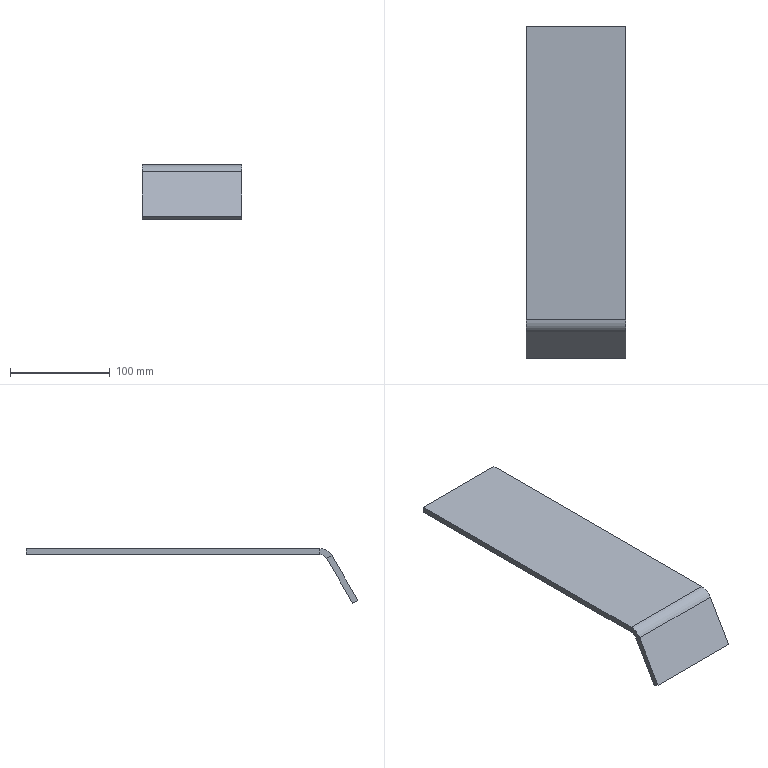Part | SolidWorks | features FlatPattern 1, SMBaseFlange 1, SheetMetal 1 | 1 solid | 14 faces | box 100 x 332 x 54.962 mm | volume 214412 mm3 | plane 12 | cylinder 2 | commonest cylinder face diameters 16 x1 28 x1
STEP:
#1=CARTESIAN_POINT('',(100.,8.083,0.));
#2=VERTEX_POINT('',#1);
#3=CARTESIAN_POINT('',(100.,8.083,-6.));
#4=VERTEX_POINT('',#3);
#5=CARTESIAN_POINT('',(100.,8.083,0.));
#6=DIRECTION('',(0.,0.,-1.));
#7=VECTOR('',#6,1000.);
#8=LINE('',#5,#7);
#9=EDGE_CURVE('',#2,#4,#8,.T.);
#10=ORIENTED_EDGE('',*,*,#9,.F.);
#11=CARTESIAN_POINT('',(100.,-4.041,-7.));
#12=VERTEX_POINT('',#11);
#13=CARTESIAN_POINT('',(100.,8.083,-14.));
#14=DIRECTION('',(1.,0.,0.));
#15=DIRECTION('',(0.,0.,1.));
#16=AXIS2_PLACEMENT_3D('',#13,#14,#15);
#17=CIRCLE('',#16,14.);
#18=EDGE_CURVE('',#2,#12,#17,.T.);
#19=ORIENTED_EDGE('',*,*,#18,.T.);
#20=CARTESIAN_POINT('',(100.,1.155,-10.));
#21=VERTEX_POINT('',#20);
#22=CARTESIAN_POINT('',(100.,1.155,-10.));
#23=DIRECTION('',(0.,-0.866,0.5));
#24=VECTOR('',#23,1000.);
#25=LINE('',#22,#24);
#26=EDGE_CURVE('',#21,#12,#25,.T.);
#27=ORIENTED_EDGE('',*,*,#26,.F.);
#28=CARTESIAN_POINT('',(100.,8.083,-14.));
#29=DIRECTION('',(1.,0.,0.));
#30=DIRECTION('',(0.,0.,-1.));
#31=AXIS2_PLACEMENT_3D('',#28,#29,#30);
#32=CIRCLE('',#31,8.);
#33=EDGE_CURVE('',#4,#21,#32,.T.);
#34=ORIENTED_EDGE('',*,*,#33,.F.);
#35=EDGE_LOOP('',(#10,#19,#27,#34));
#36=FACE_OUTER_BOUND('',#35,.T.);
#37=CARTESIAN_POINT('',(100.,8.083,0.));
#38=DIRECTION('',(1.,0.,0.));
#39=DIRECTION('',(0.,0.,-1.));
#40=AXIS2_PLACEMENT_3D('',#37,#38,#39);
#41=PLANE('',#40);
#42=ADVANCED_FACE('',(#36),#41,.T.);
#43=CARTESIAN_POINT('',(100.,302.,0.));
#44=VERTEX_POINT('',#43);
#45=CARTESIAN_POINT('',(100.,0.,0.));
#46=DIRECTION('',(0.,-1.,0.));
#47=VECTOR('',#46,1000.);
#48=LINE('',#45,#47);
#49=EDGE_CURVE('',#44,#2,#48,.T.);
#50=ORIENTED_EDGE('',*,*,#49,.T.);
#51=ORIENTED_EDGE('',*,*,#9,.T.);
#52=CARTESIAN_POINT('',(100.,302.,-6.));
#53=VERTEX_POINT('',#52);
#54=CARTESIAN_POINT('',(100.,0.,-6.));
#55=DIRECTION('',(0.,-1.,0.));
#56=VECTOR('',#55,1000.);
#57=LINE('',#54,#56);
#58=EDGE_CURVE('',#53,#4,#57,.T.);
#59=ORIENTED_EDGE('',*,*,#58,.F.);
#60=CARTESIAN_POINT('',(100.,302.,0.));
#61=DIRECTION('',(0.,0.,-1.));
#62=VECTOR('',#61,1000.);
#63=LINE('',#60,#62);
#64=EDGE_CURVE('',#44,#53,#63,.T.);
#65=ORIENTED_EDGE('',*,*,#64,.F.);
#66=EDGE_LOOP('',(#50,#51,#59,#65));
#67=FACE_OUTER_BOUND('',#66,.T.);
#68=CARTESIAN_POINT('',(100.,1.155,-10.));
#69=DIRECTION('',(1.,0.,0.));
#70=DIRECTION('',(0.,0.,-1.));
#71=AXIS2_PLACEMENT_3D('',#68,#69,#70);
#72=PLANE('',#71);
#73=ADVANCED_FACE('',(#67),#72,.T.);
#74=CARTESIAN_POINT('',(0.,-4.041,-7.));
#75=VERTEX_POINT('',#74);
#76=CARTESIAN_POINT('',(0.,1.155,-10.));
#77=VERTEX_POINT('',#76);
#78=CARTESIAN_POINT('',(0.,-4.041,-7.));
#79=DIRECTION('',(0.,0.866,-0.5));
#80=VECTOR('',#79,1000.);
#81=LINE('',#78,#80);
#82=EDGE_CURVE('',#75,#77,#81,.T.);
#83=ORIENTED_EDGE('',*,*,#82,.F.);
#84=CARTESIAN_POINT('',(0.,8.083,0.));
#85=VERTEX_POINT('',#84);
#86=CARTESIAN_POINT('',(0.,8.083,-14.));
#87=DIRECTION('',(1.,0.,0.));
#88=DIRECTION('',(0.,0.,1.));
#89=AXIS2_PLACEMENT_3D('',#86,#87,#88);
#90=CIRCLE('',#89,14.);
#91=EDGE_CURVE('',#85,#75,#90,.T.);
#92=ORIENTED_EDGE('',*,*,#91,.F.);
#93=CARTESIAN_POINT('',(0.,8.083,-6.));
#94=VERTEX_POINT('',#93);
#95=CARTESIAN_POINT('',(0.,8.083,-6.));
#96=DIRECTION('',(0.,0.,1.));
#97=VECTOR('',#96,1000.);
#98=LINE('',#95,#97);
#99=EDGE_CURVE('',#94,#85,#98,.T.);
#100=ORIENTED_EDGE('',*,*,#99,.F.);
#101=CARTESIAN_POINT('',(0.,8.083,-14.));
#102=DIRECTION('',(1.,0.,0.));
#103=DIRECTION('',(0.,0.,-1.));
#104=AXIS2_PLACEMENT_3D('',#101,#102,#103);
#105=CIRCLE('',#104,8.);
#106=EDGE_CURVE('',#94,#77,#105,.T.);
#107=ORIENTED_EDGE('',*,*,#106,.T.);
#108=EDGE_LOOP('',(#83,#92,#100,#107));
#109=FACE_OUTER_BOUND('',#108,.T.);
#110=CARTESIAN_POINT('',(0.,-4.041,-7.));
#111=DIRECTION('',(-1.,0.,0.));
#112=DIRECTION('',(0.,0.,1.));
#113=AXIS2_PLACEMENT_3D('',#110,#111,#112);
#114=PLANE('',#113);
#115=ADVANCED_FACE('',(#109),#114,.T.);
#116=CARTESIAN_POINT('',(0.,-30.,-51.962));
#117=VERTEX_POINT('',#116);
#118=CARTESIAN_POINT('',(0.,0.,0.));
#119=DIRECTION('',(0.,-0.5,-0.866));
#120=VECTOR('',#119,1000.);
#121=LINE('',#118,#120);
#122=EDGE_CURVE('',#75,#117,#121,.T.);
#123=ORIENTED_EDGE('',*,*,#122,.F.);
#124=ORIENTED_EDGE('',*,*,#82,.T.);
#125=CARTESIAN_POINT('',(0.,-24.804,-54.962));
#126=VERTEX_POINT('',#125);
#127=CARTESIAN_POINT('',(0.,5.196,-3.));
#128=DIRECTION('',(0.,-0.5,-0.866));
#129=VECTOR('',#128,1000.);
#130=LINE('',#127,#129);
#131=EDGE_CURVE('',#77,#126,#130,.T.);
#132=ORIENTED_EDGE('',*,*,#131,.T.);
#133=CARTESIAN_POINT('',(0.,-24.804,-54.962));
#134=DIRECTION('',(0.,-0.866,0.5));
#135=VECTOR('',#134,1000.);
#136=LINE('',#133,#135);
#137=EDGE_CURVE('',#126,#117,#136,.T.);
#138=ORIENTED_EDGE('',*,*,#137,.T.);
#139=EDGE_LOOP('',(#123,#124,#132,#138));
#140=FACE_OUTER_BOUND('',#139,.T.);
#141=CARTESIAN_POINT('',(0.,8.083,-6.));
#142=DIRECTION('',(-1.,0.,0.));
#143=DIRECTION('',(0.,0.,1.));
#144=AXIS2_PLACEMENT_3D('',#141,#142,#143);
#145=PLANE('',#144);
#146=ADVANCED_FACE('',(#140),#145,.T.);
#147=ORIENTED_EDGE('',*,*,#122,.T.);
#148=CARTESIAN_POINT('',(100.,-30.,-51.962));
#149=VERTEX_POINT('',#148);
#150=CARTESIAN_POINT('',(100.,-30.,-51.962));
#151=DIRECTION('',(-1.,0.,0.));
#152=VECTOR('',#151,1000.);
#153=LINE('',#150,#152);
#154=EDGE_CURVE('',#149,#117,#153,.T.);
#155=ORIENTED_EDGE('',*,*,#154,.F.);
#156=CARTESIAN_POINT('',(100.,0.,0.));
#157=DIRECTION('',(0.,-0.5,-0.866));
#158=VECTOR('',#157,1000.);
#159=LINE('',#156,#158);
#160=EDGE_CURVE('',#12,#149,#159,.T.);
#161=ORIENTED_EDGE('',*,*,#160,.F.);
#162=CARTESIAN_POINT('',(100.,-4.041,-7.));
#163=DIRECTION('',(-1.,0.,0.));
#164=VECTOR('',#163,1000.);
#165=LINE('',#162,#164);
#166=EDGE_CURVE('',#12,#75,#165,.T.);
#167=ORIENTED_EDGE('',*,*,#166,.T.);
#168=EDGE_LOOP('',(#147,#155,#161,#167));
#169=FACE_OUTER_BOUND('',#168,.T.);
#170=CARTESIAN_POINT('',(100.,0.,0.));
#171=DIRECTION('',(0.,0.866,-0.5));
#172=DIRECTION('',(0.,0.5,0.866));
#173=AXIS2_PLACEMENT_3D('',#170,#171,#172);
#174=PLANE('',#173);
#175=ADVANCED_FACE('',(#169),#174,.F.);
#176=ORIENTED_EDGE('',*,*,#137,.F.);
#177=CARTESIAN_POINT('',(100.,-24.804,-54.962));
#178=VERTEX_POINT('',#177);
#179=CARTESIAN_POINT('',(100.,-24.804,-54.962));
#180=DIRECTION('',(-1.,0.,0.));
#181=VECTOR('',#180,1000.);
#182=LINE('',#179,#181);
#183=EDGE_CURVE('',#178,#126,#182,.T.);
#184=ORIENTED_EDGE('',*,*,#183,.F.);
#185=CARTESIAN_POINT('',(100.,-24.804,-54.962));
#186=DIRECTION('',(0.,-0.866,0.5));
#187=VECTOR('',#186,1000.);
#188=LINE('',#185,#187);
#189=EDGE_CURVE('',#178,#149,#188,.T.);
#190=ORIENTED_EDGE('',*,*,#189,.T.);
#191=ORIENTED_EDGE('',*,*,#154,.T.);
#192=EDGE_LOOP('',(#176,#184,#190,#191));
#193=FACE_OUTER_BOUND('',#192,.T.);
#194=CARTESIAN_POINT('',(100.,-24.804,-54.962));
#195=DIRECTION('',(0.,-0.5,-0.866));
#196=DIRECTION('',(0.,0.866,-0.5));
#197=AXIS2_PLACEMENT_3D('',#194,#195,#196);
#198=PLANE('',#197);
#199=ADVANCED_FACE('',(#193),#198,.T.);
#200=ORIENTED_EDGE('',*,*,#131,.F.);
#201=CARTESIAN_POINT('',(100.,1.155,-10.));
#202=DIRECTION('',(-1.,0.,0.));
#203=VECTOR('',#202,1000.);
#204=LINE('',#201,#203);
#205=EDGE_CURVE('',#21,#77,#204,.T.);
#206=ORIENTED_EDGE('',*,*,#205,.F.);
#207=CARTESIAN_POINT('',(100.,5.196,-3.));
#208=DIRECTION('',(0.,-0.5,-0.866));
#209=VECTOR('',#208,1000.);
#210=LINE('',#207,#209);
#211=EDGE_CURVE('',#21,#178,#210,.T.);
#212=ORIENTED_EDGE('',*,*,#211,.T.);
#213=ORIENTED_EDGE('',*,*,#183,.T.);
#214=EDGE_LOOP('',(#200,#206,#212,#213));
#215=FACE_OUTER_BOUND('',#214,.T.);
#216=CARTESIAN_POINT('',(100.,5.196,-3.));
#217=DIRECTION('',(0.,0.866,-0.5));
#218=DIRECTION('',(0.,0.5,0.866));
#219=AXIS2_PLACEMENT_3D('',#216,#217,#218);
#220=PLANE('',#219);
#221=ADVANCED_FACE('',(#215),#220,.T.);
#222=ORIENTED_EDGE('',*,*,#106,.F.);
#223=CARTESIAN_POINT('',(100.,8.083,-6.));
#224=DIRECTION('',(-1.,0.,0.));
#225=VECTOR('',#224,1000.);
#226=LINE('',#223,#225);
#227=EDGE_CURVE('',#4,#94,#226,.T.);
#228=ORIENTED_EDGE('',*,*,#227,.F.);
#229=ORIENTED_EDGE('',*,*,#33,.T.);
#230=ORIENTED_EDGE('',*,*,#205,.T.);
#231=EDGE_LOOP('',(#222,#228,#229,#230));
#232=FACE_OUTER_BOUND('',#231,.T.);
#233=CARTESIAN_POINT('',(100.,8.083,-14.));
#234=DIRECTION('',(-1.,0.,0.));
#235=DIRECTION('',(0.,0.,1.));
#236=AXIS2_PLACEMENT_3D('',#233,#234,#235);
#237=CYLINDRICAL_SURFACE('',#236,8.);
#238=ADVANCED_FACE('',(#232),#237,.F.);
#239=CARTESIAN_POINT('',(0.,302.,-6.));
#240=VERTEX_POINT('',#239);
#241=CARTESIAN_POINT('',(0.,0.,-6.));
#242=DIRECTION('',(0.,-1.,0.));
#243=VECTOR('',#242,1000.);
#244=LINE('',#241,#243);
#245=EDGE_CURVE('',#240,#94,#244,.T.);
#246=ORIENTED_EDGE('',*,*,#245,.F.);
#247=CARTESIAN_POINT('',(100.,302.,-6.));
#248=DIRECTION('',(-1.,0.,0.));
#249=VECTOR('',#248,1000.);
#250=LINE('',#247,#249);
#251=EDGE_CURVE('',#53,#240,#250,.T.);
#252=ORIENTED_EDGE('',*,*,#251,.F.);
#253=ORIENTED_EDGE('',*,*,#58,.T.);
#254=ORIENTED_EDGE('',*,*,#227,.T.);
#255=EDGE_LOOP('',(#246,#252,#253,#254));
#256=FACE_OUTER_BOUND('',#255,.T.);
#257=CARTESIAN_POINT('',(100.,0.,-6.));
#258=DIRECTION('',(0.,0.,-1.));
#259=DIRECTION('',(-1.,0.,0.));
#260=AXIS2_PLACEMENT_3D('',#257,#258,#259);
#261=PLANE('',#260);
#262=ADVANCED_FACE('',(#256),#261,.T.);
#263=CARTESIAN_POINT('',(0.,302.,0.));
#264=VERTEX_POINT('',#263);
#265=CARTESIAN_POINT('',(0.,302.,0.));
#266=DIRECTION('',(0.,0.,-1.));
#267=VECTOR('',#266,1000.);
#268=LINE('',#265,#267);
#269=EDGE_CURVE('',#264,#240,#268,.T.);
#270=ORIENTED_EDGE('',*,*,#269,.F.);
#271=CARTESIAN_POINT('',(100.,302.,0.));
#272=DIRECTION('',(-1.,0.,0.));
#273=VECTOR('',#272,1000.);
#274=LINE('',#271,#273);
#275=EDGE_CURVE('',#44,#264,#274,.T.);
#276=ORIENTED_EDGE('',*,*,#275,.F.);
#277=ORIENTED_EDGE('',*,*,#64,.T.);
#278=ORIENTED_EDGE('',*,*,#251,.T.);
#279=EDGE_LOOP('',(#270,#276,#277,#278));
#280=FACE_OUTER_BOUND('',#279,.T.);
#281=CARTESIAN_POINT('',(100.,302.,0.));
#282=DIRECTION('',(0.,1.,0.));
#283=DIRECTION('',(0.,0.,1.));
#284=AXIS2_PLACEMENT_3D('',#281,#282,#283);
#285=PLANE('',#284);
#286=ADVANCED_FACE('',(#280),#285,.T.);
#287=CARTESIAN_POINT('',(0.,0.,0.));
#288=DIRECTION('',(0.,-1.,0.));
#289=VECTOR('',#288,1000.);
#290=LINE('',#287,#289);
#291=EDGE_CURVE('',#264,#85,#290,.T.);
#292=ORIENTED_EDGE('',*,*,#291,.T.);
#293=CARTESIAN_POINT('',(100.,8.083,0.));
#294=DIRECTION('',(-1.,0.,0.));
#295=VECTOR('',#294,1000.);
#296=LINE('',#293,#295);
#297=EDGE_CURVE('',#2,#85,#296,.T.);
#298=ORIENTED_EDGE('',*,*,#297,.F.);
#299=ORIENTED_EDGE('',*,*,#49,.F.);
#300=ORIENTED_EDGE('',*,*,#275,.T.);
#301=EDGE_LOOP('',(#292,#298,#299,#300));
#302=FACE_OUTER_BOUND('',#301,.T.);
#303=CARTESIAN_POINT('',(100.,0.,0.));
#304=DIRECTION('',(0.,0.,-1.));
#305=DIRECTION('',(-1.,0.,0.));
#306=AXIS2_PLACEMENT_3D('',#303,#304,#305);
#307=PLANE('',#306);
#308=ADVANCED_FACE('',(#302),#307,.F.);
#309=ORIENTED_EDGE('',*,*,#91,.T.);
#310=ORIENTED_EDGE('',*,*,#166,.F.);
#311=ORIENTED_EDGE('',*,*,#18,.F.);
#312=ORIENTED_EDGE('',*,*,#297,.T.);
#313=EDGE_LOOP('',(#309,#310,#311,#312));
#314=FACE_OUTER_BOUND('',#313,.T.);
#315=CARTESIAN_POINT('',(100.,8.083,-14.));
#316=DIRECTION('',(-1.,0.,0.));
#317=DIRECTION('',(0.,0.,1.));
#318=AXIS2_PLACEMENT_3D('',#315,#316,#317);
#319=CYLINDRICAL_SURFACE('',#318,14.);
#320=ADVANCED_FACE('',(#314),#319,.T.);
#321=ORIENTED_EDGE('',*,*,#160,.T.);
#322=ORIENTED_EDGE('',*,*,#189,.F.);
#323=ORIENTED_EDGE('',*,*,#211,.F.);
#324=ORIENTED_EDGE('',*,*,#26,.T.);
#325=EDGE_LOOP('',(#321,#322,#323,#324));
#326=FACE_OUTER_BOUND('',#325,.T.);
#327=CARTESIAN_POINT('',(100.,8.083,-14.));
#328=DIRECTION('',(1.,0.,0.));
#329=DIRECTION('',(0.,0.,-1.));
#330=AXIS2_PLACEMENT_3D('',#327,#328,#329);
#331=PLANE('',#330);
#332=ADVANCED_FACE('',(#326),#331,.T.);
#333=ORIENTED_EDGE('',*,*,#245,.T.);
#334=ORIENTED_EDGE('',*,*,#99,.T.);
#335=ORIENTED_EDGE('',*,*,#291,.F.);
#336=ORIENTED_EDGE('',*,*,#269,.T.);
#337=EDGE_LOOP('',(#333,#334,#335,#336));
#338=FACE_OUTER_BOUND('',#337,.T.);
#339=CARTESIAN_POINT('',(0.,8.083,-14.));
#340=DIRECTION('',(1.,0.,0.));
#341=DIRECTION('',(0.,0.,-1.));
#342=AXIS2_PLACEMENT_3D('',#339,#340,#341);
#343=PLANE('',#342);
#344=ADVANCED_FACE('',(#338),#343,.F.);
#345=CLOSED_SHELL('',(#42,#73,#115,#146,#175,#199,#221,#238,#262,#286,#308,#320,#332,#344));
#346=MANIFOLD_SOLID_BREP('',#345);
#347=CARTESIAN_POINT('',(0.,0.,0.));
#348=DIRECTION('',(0.,0.,1.));
#349=DIRECTION('',(1.,0.,0.));
#350=AXIS2_PLACEMENT_3D('',#347,#348,#349);
#351=(LENGTH_UNIT()NAMED_UNIT(*)SI_UNIT(.MILLI.,.METRE.));
#352=UNCERTAINTY_MEASURE_WITH_UNIT(LENGTH_MEASURE(0.00001),#351,'','');
#353=(NAMED_UNIT(*)PLANE_ANGLE_UNIT()SI_UNIT($,.RADIAN.));
#354=(NAMED_UNIT(*)SI_UNIT($,.STERADIAN.)SOLID_ANGLE_UNIT());
#355=(GEOMETRIC_REPRESENTATION_CONTEXT(3)GLOBAL_UNCERTAINTY_ASSIGNED_CONTEXT((#352))GLOBAL_UNIT_ASSIGNED_CONTEXT((#351,#353,#354))REPRESENTATION_CONTEXT('',''));
#356=ADVANCED_BREP_SHAPE_REPRESENTATION('',(#346,#350),#355);